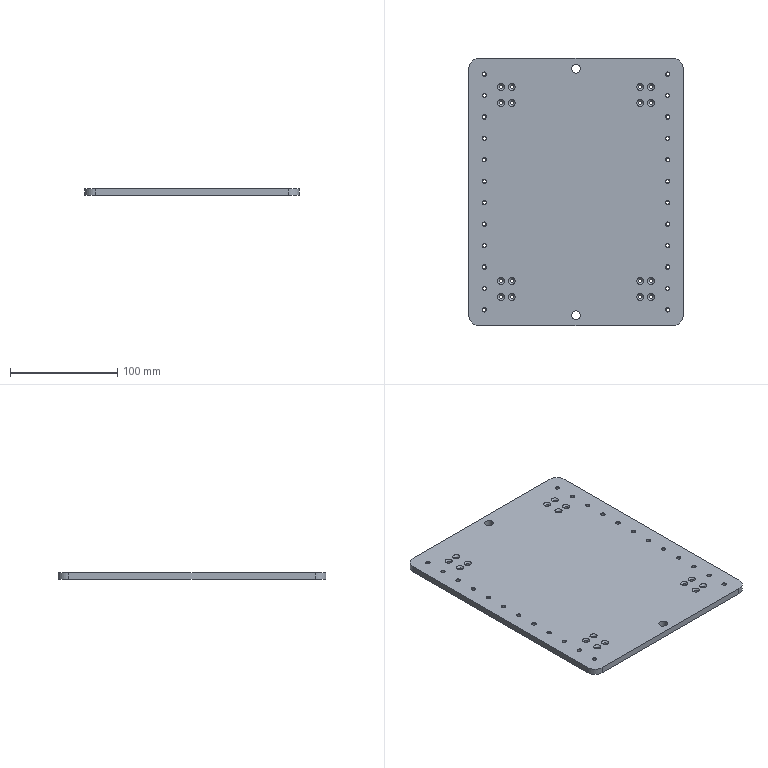Part | STEP file | JBJ-P-1014-01 | 1 solid | 92 faces | box 200 x 250 x 6 mm | volume 296472 mm3 | cylinder 46 | cone 40 | plane 6 | commonest cylinder face diameters 3.3 x24 3.4 x16 20 x4 8 x2